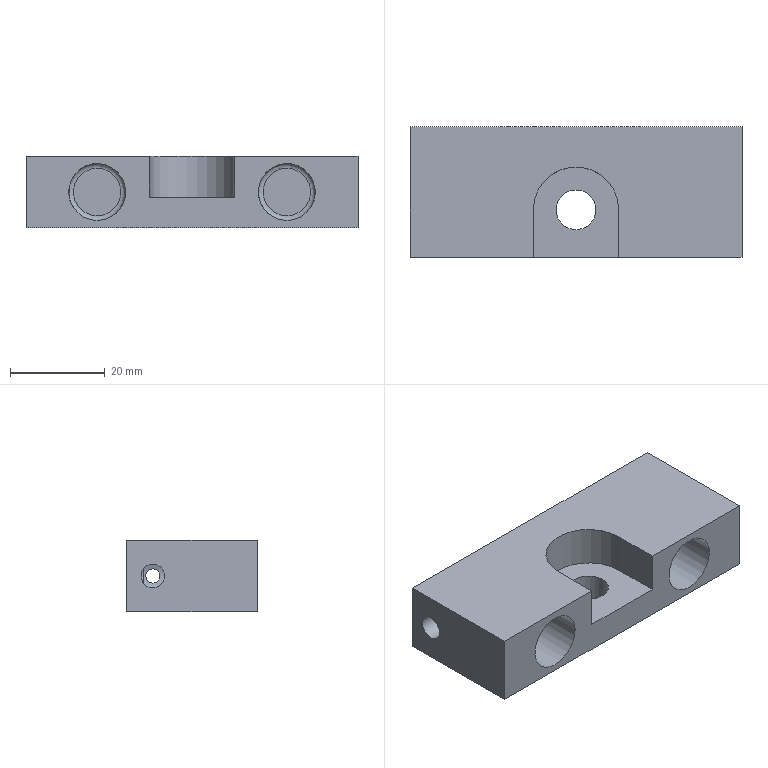NC program | NX | posted with a generic post | part box 70 x 27.5 x 15 mm
Lines 3295 to 3352 of 3352:
(PLANAR_MILL_3 , TOOL : 倒角D4-90度)
N6558 T05 M6
N6560 G53
N6562 G17 G0 G90 X-15.75 Y-38.464 B0. C0. S3000 M3
N6564 G43 Z20. H5
N6566 Z0.
N6568 G94 G1 Z-2. F800.
N6570 Y-34.999
N6572 Y-9.
N6574 G2 X-13.75 Y-7. R2.
N6576 G1 X-3.75
N6578 G3 X3.25 Y0. R7.
N6580 X-3.75 Y7. R7.
N6582 G1 X-13.75
N6584 G2 X-15.75 Y9. R2.
N6586 G1 Y35.
N6588 G2 X-13.75 Y37. R2.
N6590 G1 X13.75
N6592 G2 X15.75 Y35. R2.
N6594 G1 Y-35.
N6596 G2 X13.75 Y-37. R2.
N6598 G1 X-13.749
N6600 X-17.214
N6602 Z0.
N6604 G0 Z20.
(PLANAR_MILL_3_COPY , TOOL : 倒角D4-90度)
N6606 X-2.75 Y0.663
N6608 Z-8.6
N6610 G1 Z-10.6
N6612 Y1.2
N6614 G3 X-3.75 Y2.2 R1.
N6616 X-5.95 Y0. R2.2
N6618 X-3.75 Y2.2 R-2.2
N6620 X-4.75 Y1.2 R1.
N6622 G1 Y0.663
N6624 Z-8.6
N6626 G0 Z20.
N6628 M5
(PLANAR_MILL_COPY_COPY , TOOL : D50面刀)
N6630 T01 M6
N6632 G53
N6634 G17 G0 G90 X-0.05 Y-65. B0. C0. S2500 M3
N6636 G43 Z20. H1
N6638 Z3.
N6640 G94 G1 Z0. F600.
N6642 Y-35.
N6644 Y35.
N6646 Y65.
N6648 Z3.
N6650 G0 Z20.
N6652 M5
N6654 M2